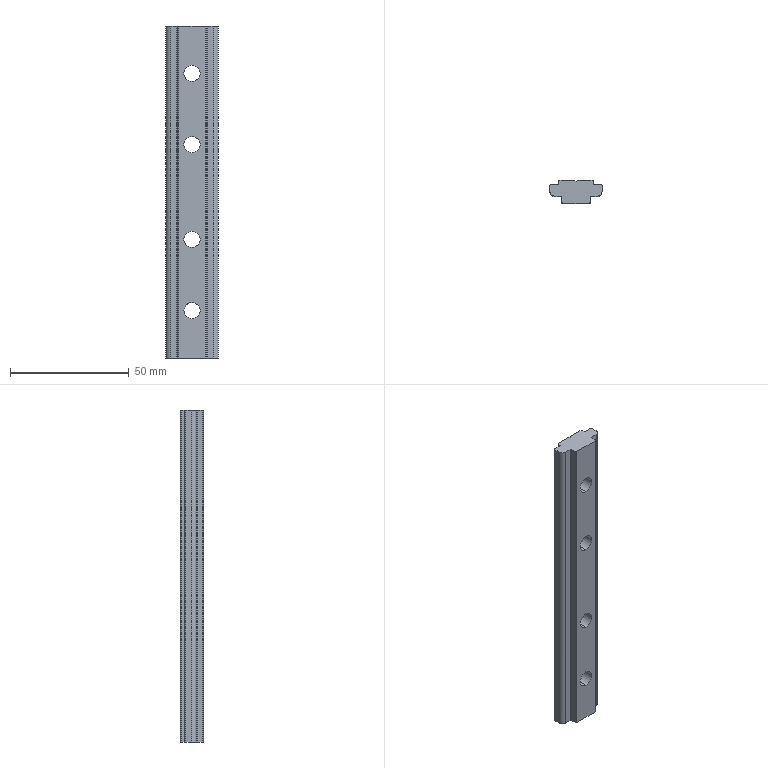Part | STEP file | 46A-01006CC13 | 1 solid | 45 faces | box 22 x 9.7 x 140 mm | volume 22186 mm3 | plane 25 | cylinder 20 | commonest cylinder face diameters 1 x8 6.8 x8 0.4 x2 4 x2